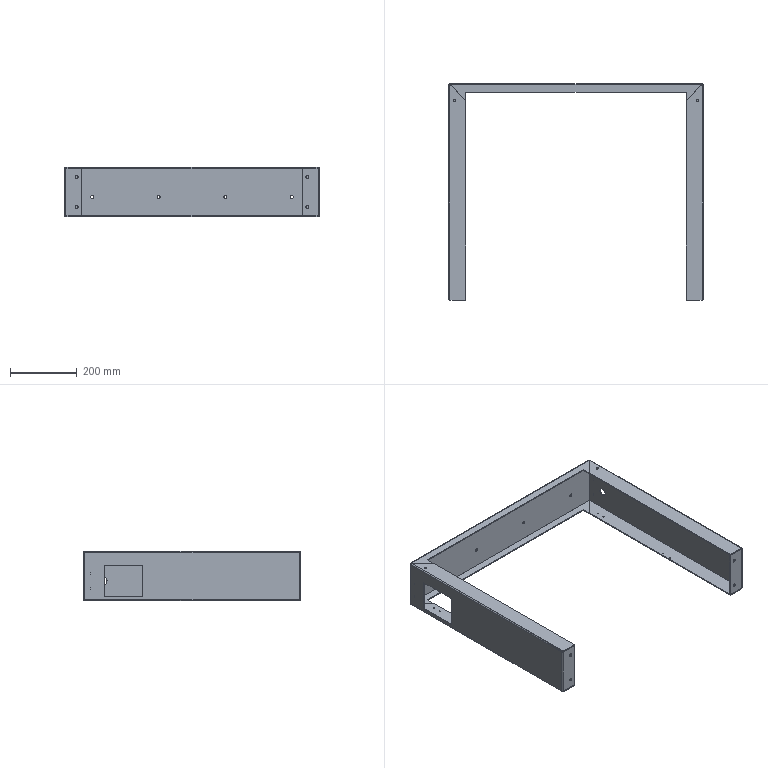Part | STEP file | HESS-408-70-15W-W-17-outer case lower support 1 | 1 solid | 144 faces | box 763 x 650 x 150 mm | volume 1372071 mm3 | plane 82 | cylinder 54 | spline 8 | commonest cylinder face diameters 9 x16 3.2 x12 0.2 x10 6.2 x10 6.8 x4 22 x2